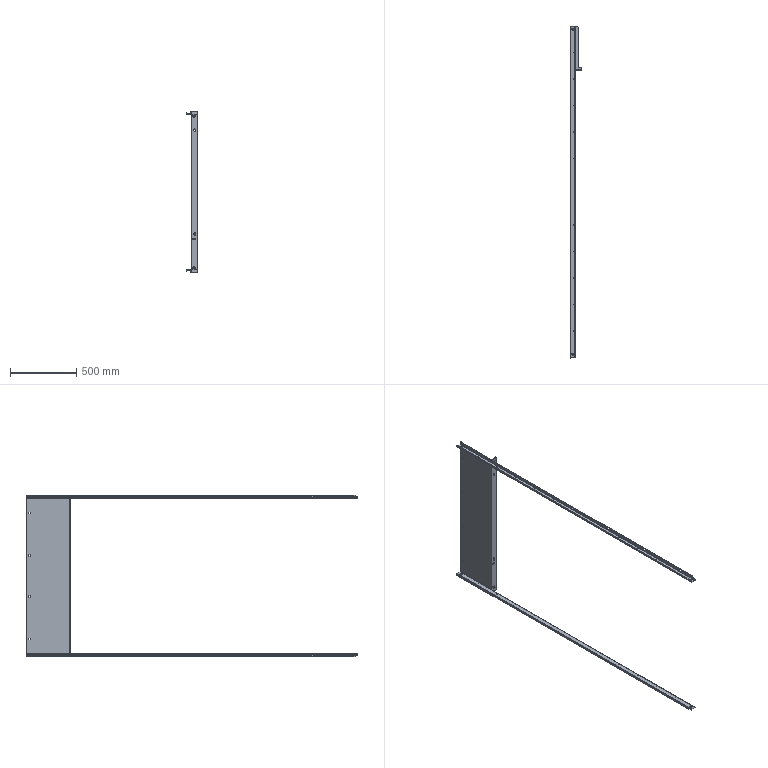Part | SolidWorks | 5 solids | 346 faces | box 90 x 2502 x 1221 mm | volume 1703214 mm3 | plane 174 | cylinder 172 | commonest cylinder face diameters 8 x80 4.2 x40 10 x26 2 x11 11 x8 4 x4